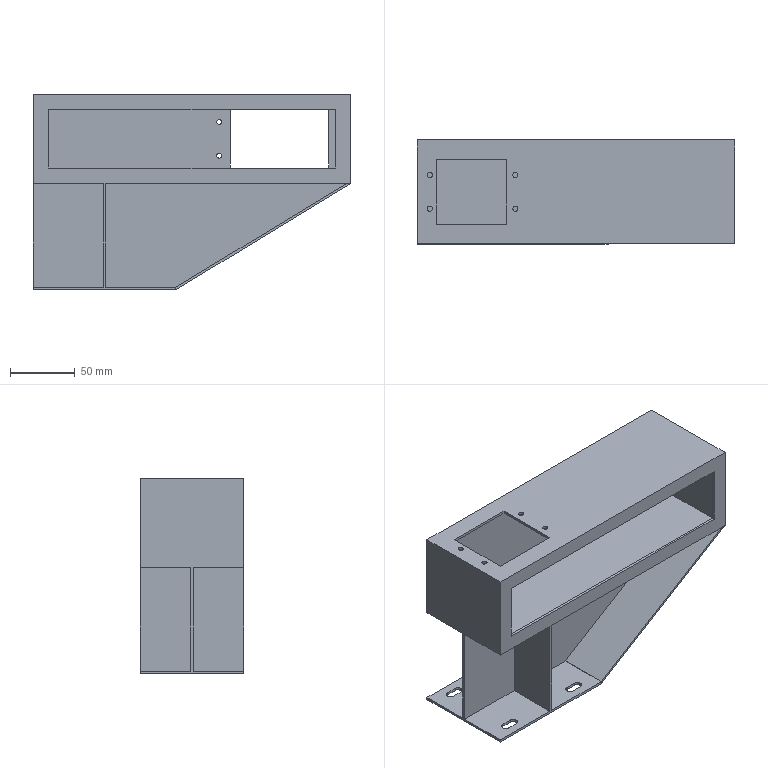Part | SolidWorks | features BaseBody 2 | 2 solids | 83 faces | box 245 x 80 x 151 mm | volume 206222 mm3 | plane 55 | cylinder 28 | commonest cylinder face diameters 4 x16 6.5 x12